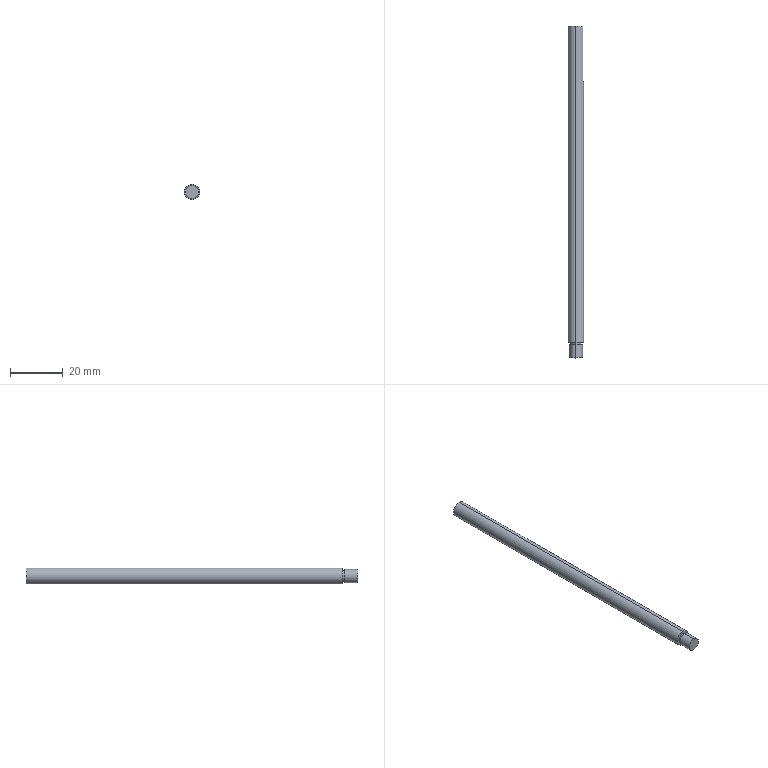Part | STEP file | 1 solid | 12 faces | box 6 x 126 x 6 mm | volume 3480 mm3 | cylinder 6 | plane 6 | commonest cylinder face diameters 4 x2 5 x2 6 x2
STEP:
#1=CARTESIAN_POINT('',(0.,0.,0.));
#2=DIRECTION('',(0.,0.,1.));
#3=DIRECTION('',(1.,0.,0.));
#4=AXIS2_PLACEMENT_3D('',#1,#2,#3);
#5=CARTESIAN_POINT('',(0.,-6.,-2.5));
#6=VERTEX_POINT('',#5);
#7=CARTESIAN_POINT('',(0.,-6.,2.5));
#8=VERTEX_POINT('',#7);
#9=CARTESIAN_POINT('',(0.,-6.,0.));
#10=DIRECTION('',(0.,-1.,0.));
#11=DIRECTION('',(0.,0.,-1.));
#12=AXIS2_PLACEMENT_3D('',#9,#10,#11);
#13=CIRCLE('',#12,2.5);
#14=CARTESIAN_POINT('',(0.,-6.,0.));
#15=DIRECTION('',(0.,1.,0.));
#16=DIRECTION('',(0.,0.,1.));
#17=AXIS2_PLACEMENT_3D('',#14,#15,#16);
#18=CYLINDRICAL_SURFACE('',#17,2.5);
#19=CARTESIAN_POINT('',(3.142,0.));
#20=DIRECTION('',(-1.,0.));
#21=VECTOR('',#20,1.);
#22=LINE('',#19,#21);
#23=(GEOMETRIC_REPRESENTATION_CONTEXT(2)PARAMETRIC_REPRESENTATION_CONTEXT()REPRESENTATION_CONTEXT('',''));
#24=DEFINITIONAL_REPRESENTATION('',(#22),#23);
#25=PCURVE('',#18,#24);
#26=CARTESIAN_POINT('',(0.,-6.,0.));
#27=DIRECTION('',(0.,-1.,0.));
#28=DIRECTION('',(0.,0.,-1.));
#29=AXIS2_PLACEMENT_3D('',#26,#27,#28);
#30=PLANE('',#29);
#31=CARTESIAN_POINT('',(0.,0.));
#32=DIRECTION('',(1.,0.));
#33=AXIS2_PLACEMENT_2D('',#31,#32);
#34=CIRCLE('',#33,2.5);
#35=(GEOMETRIC_REPRESENTATION_CONTEXT(2)PARAMETRIC_REPRESENTATION_CONTEXT()REPRESENTATION_CONTEXT('',''));
#36=DEFINITIONAL_REPRESENTATION('',(#34),#35);
#37=PCURVE('',#30,#36);
#38=SURFACE_CURVE('',#13,(#25,#37),.PCURVE_S1.);
#39=EDGE_CURVE('',#6,#8,#38,.T.);
#40=ORIENTED_EDGE('',*,*,#39,.F.);
#41=CARTESIAN_POINT('',(0.,-1.,-2.5));
#42=VERTEX_POINT('',#41);
#43=CARTESIAN_POINT('',(0.,-6.,-2.5));
#44=DIRECTION('',(0.,1.,0.));
#45=VECTOR('',#44,1.);
#46=LINE('',#43,#45);
#47=CARTESIAN_POINT('',(3.142,0.));
#48=DIRECTION('',(0.,1.));
#49=VECTOR('',#48,1.);
#50=LINE('',#47,#49);
#51=(GEOMETRIC_REPRESENTATION_CONTEXT(2)PARAMETRIC_REPRESENTATION_CONTEXT()REPRESENTATION_CONTEXT('',''));
#52=DEFINITIONAL_REPRESENTATION('',(#50),#51);
#53=PCURVE('',#18,#52);
#54=CARTESIAN_POINT('',(0.,-6.,0.));
#55=DIRECTION('',(0.,1.,0.));
#56=DIRECTION('',(0.,0.,1.));
#57=AXIS2_PLACEMENT_3D('',#54,#55,#56);
#58=CYLINDRICAL_SURFACE('',#57,2.5);
#59=CARTESIAN_POINT('',(3.142,0.));
#60=DIRECTION('',(0.,1.));
#61=VECTOR('',#60,1.);
#62=LINE('',#59,#61);
#63=(GEOMETRIC_REPRESENTATION_CONTEXT(2)PARAMETRIC_REPRESENTATION_CONTEXT()REPRESENTATION_CONTEXT('',''));
#64=DEFINITIONAL_REPRESENTATION('',(#62),#63);
#65=PCURVE('',#58,#64);
#66=SURFACE_CURVE('',#46,(#53,#65),.PCURVE_S1.);
#67=EDGE_CURVE('',#6,#42,#66,.T.);
#68=ORIENTED_EDGE('',*,*,#67,.T.);
#69=CARTESIAN_POINT('',(0.,-1.,2.5));
#70=VERTEX_POINT('',#69);
#71=CARTESIAN_POINT('',(0.,-1.,0.));
#72=DIRECTION('',(0.,-1.,0.));
#73=DIRECTION('',(0.,0.,-1.));
#74=AXIS2_PLACEMENT_3D('',#71,#72,#73);
#75=CIRCLE('',#74,2.5);
#76=CARTESIAN_POINT('',(3.142,5.));
#77=DIRECTION('',(-1.,0.));
#78=VECTOR('',#77,1.);
#79=LINE('',#76,#78);
#80=(GEOMETRIC_REPRESENTATION_CONTEXT(2)PARAMETRIC_REPRESENTATION_CONTEXT()REPRESENTATION_CONTEXT('',''));
#81=DEFINITIONAL_REPRESENTATION('',(#79),#80);
#82=PCURVE('',#18,#81);
#83=CARTESIAN_POINT('',(0.,-1.,0.));
#84=DIRECTION('',(0.,-1.,0.));
#85=DIRECTION('',(0.,0.,-1.));
#86=AXIS2_PLACEMENT_3D('',#83,#84,#85);
#87=PLANE('',#86);
#88=CARTESIAN_POINT('',(0.,0.));
#89=DIRECTION('',(1.,0.));
#90=AXIS2_PLACEMENT_2D('',#88,#89);
#91=CIRCLE('',#90,2.5);
#92=(GEOMETRIC_REPRESENTATION_CONTEXT(2)PARAMETRIC_REPRESENTATION_CONTEXT()REPRESENTATION_CONTEXT('',''));
#93=DEFINITIONAL_REPRESENTATION('',(#91),#92);
#94=PCURVE('',#87,#93);
#95=SURFACE_CURVE('',#75,(#82,#94),.PCURVE_S1.);
#96=EDGE_CURVE('',#42,#70,#95,.T.);
#97=ORIENTED_EDGE('',*,*,#96,.T.);
#98=CARTESIAN_POINT('',(0.,-6.,2.5));
#99=DIRECTION('',(0.,1.,0.));
#100=VECTOR('',#99,1.);
#101=LINE('',#98,#100);
#102=CARTESIAN_POINT('',(0.,0.));
#103=DIRECTION('',(0.,1.));
#104=VECTOR('',#103,1.);
#105=LINE('',#102,#104);
#106=(GEOMETRIC_REPRESENTATION_CONTEXT(2)PARAMETRIC_REPRESENTATION_CONTEXT()REPRESENTATION_CONTEXT('',''));
#107=DEFINITIONAL_REPRESENTATION('',(#105),#106);
#108=PCURVE('',#18,#107);
#109=CARTESIAN_POINT('',(6.283,0.));
#110=DIRECTION('',(0.,1.));
#111=VECTOR('',#110,1.);
#112=LINE('',#109,#111);
#113=(GEOMETRIC_REPRESENTATION_CONTEXT(2)PARAMETRIC_REPRESENTATION_CONTEXT()REPRESENTATION_CONTEXT('',''));
#114=DEFINITIONAL_REPRESENTATION('',(#112),#113);
#115=PCURVE('',#58,#114);
#116=SURFACE_CURVE('',#101,(#108,#115),.PCURVE_S1.);
#117=EDGE_CURVE('',#8,#70,#116,.T.);
#118=ORIENTED_EDGE('',*,*,#117,.F.);
#119=EDGE_LOOP('',(#40,#68,#97,#118));
#120=FACE_BOUND('',#119,.T.);
#121=ADVANCED_FACE('',(#120),#18,.T.);
#122=CARTESIAN_POINT('',(0.,-1.,-2.));
#123=VERTEX_POINT('',#122);
#124=CARTESIAN_POINT('',(0.,-1.,2.));
#125=VERTEX_POINT('',#124);
#126=CARTESIAN_POINT('',(0.,-1.,0.));
#127=DIRECTION('',(0.,-1.,0.));
#128=DIRECTION('',(0.,0.,-1.));
#129=AXIS2_PLACEMENT_3D('',#126,#127,#128);
#130=CIRCLE('',#129,2.);
#131=CARTESIAN_POINT('',(0.,-1.,0.));
#132=DIRECTION('',(0.,1.,0.));
#133=DIRECTION('',(0.,0.,1.));
#134=AXIS2_PLACEMENT_3D('',#131,#132,#133);
#135=CYLINDRICAL_SURFACE('',#134,2.);
#136=CARTESIAN_POINT('',(3.142,0.));
#137=DIRECTION('',(-1.,0.));
#138=VECTOR('',#137,1.);
#139=LINE('',#136,#138);
#140=(GEOMETRIC_REPRESENTATION_CONTEXT(2)PARAMETRIC_REPRESENTATION_CONTEXT()REPRESENTATION_CONTEXT('',''));
#141=DEFINITIONAL_REPRESENTATION('',(#139),#140);
#142=PCURVE('',#135,#141);
#143=CARTESIAN_POINT('',(0.,0.));
#144=DIRECTION('',(1.,0.));
#145=AXIS2_PLACEMENT_2D('',#143,#144);
#146=CIRCLE('',#145,2.);
#147=(GEOMETRIC_REPRESENTATION_CONTEXT(2)PARAMETRIC_REPRESENTATION_CONTEXT()REPRESENTATION_CONTEXT('',''));
#148=DEFINITIONAL_REPRESENTATION('',(#146),#147);
#149=PCURVE('',#87,#148);
#150=SURFACE_CURVE('',#130,(#142,#149),.PCURVE_S1.);
#151=EDGE_CURVE('',#123,#125,#150,.T.);
#152=ORIENTED_EDGE('',*,*,#151,.F.);
#153=CARTESIAN_POINT('',(0.,0.,-2.));
#154=VERTEX_POINT('',#153);
#155=CARTESIAN_POINT('',(0.,-1.,-2.));
#156=DIRECTION('',(0.,1.,0.));
#157=VECTOR('',#156,1.);
#158=LINE('',#155,#157);
#159=CARTESIAN_POINT('',(3.142,0.));
#160=DIRECTION('',(0.,1.));
#161=VECTOR('',#160,1.);
#162=LINE('',#159,#161);
#163=(GEOMETRIC_REPRESENTATION_CONTEXT(2)PARAMETRIC_REPRESENTATION_CONTEXT()REPRESENTATION_CONTEXT('',''));
#164=DEFINITIONAL_REPRESENTATION('',(#162),#163);
#165=PCURVE('',#135,#164);
#166=CARTESIAN_POINT('',(0.,-1.,0.));
#167=DIRECTION('',(0.,1.,0.));
#168=DIRECTION('',(0.,0.,1.));
#169=AXIS2_PLACEMENT_3D('',#166,#167,#168);
#170=CYLINDRICAL_SURFACE('',#169,2.);
#171=CARTESIAN_POINT('',(3.142,0.));
#172=DIRECTION('',(0.,1.));
#173=VECTOR('',#172,1.);
#174=LINE('',#171,#173);
#175=(GEOMETRIC_REPRESENTATION_CONTEXT(2)PARAMETRIC_REPRESENTATION_CONTEXT()REPRESENTATION_CONTEXT('',''));
#176=DEFINITIONAL_REPRESENTATION('',(#174),#175);
#177=PCURVE('',#170,#176);
#178=SURFACE_CURVE('',#158,(#165,#177),.PCURVE_S1.);
#179=EDGE_CURVE('',#123,#154,#178,.T.);
#180=ORIENTED_EDGE('',*,*,#179,.T.);
#181=CARTESIAN_POINT('',(0.,0.,2.));
#182=VERTEX_POINT('',#181);
#183=CARTESIAN_POINT('',(0.,0.,0.));
#184=DIRECTION('',(0.,-1.,0.));
#185=DIRECTION('',(0.,0.,-1.));
#186=AXIS2_PLACEMENT_3D('',#183,#184,#185);
#187=CIRCLE('',#186,2.);
#188=CARTESIAN_POINT('',(3.142,1.));
#189=DIRECTION('',(-1.,0.));
#190=VECTOR('',#189,1.);
#191=LINE('',#188,#190);
#192=(GEOMETRIC_REPRESENTATION_CONTEXT(2)PARAMETRIC_REPRESENTATION_CONTEXT()REPRESENTATION_CONTEXT('',''));
#193=DEFINITIONAL_REPRESENTATION('',(#191),#192);
#194=PCURVE('',#135,#193);
#195=CARTESIAN_POINT('',(0.,0.,0.));
#196=DIRECTION('',(0.,1.,0.));
#197=DIRECTION('',(0.,0.,1.));
#198=AXIS2_PLACEMENT_3D('',#195,#196,#197);
#199=PLANE('',#198);
#200=CARTESIAN_POINT('',(-2.,0.));
#201=CARTESIAN_POINT('',(-2.,3.464));
#202=CARTESIAN_POINT('',(1.,1.732));
#203=CARTESIAN_POINT('',(4.,0.));
#204=CARTESIAN_POINT('',(1.,-1.732));
#205=CARTESIAN_POINT('',(-2.,-3.464));
#206=CARTESIAN_POINT('',(-2.,0.));
#207=(BOUNDED_CURVE()B_SPLINE_CURVE(2,(#200,#201,#202,#203,#204,#205,#206),.UNSPECIFIED.,.T.,.F.)B_SPLINE_CURVE_WITH_KNOTS((1,2,2,2,2,1),(-2.094,0.,2.094,4.189,6.283,8.378),.UNSPECIFIED.)CURVE()GEOMETRIC_REPRESENTATION_ITEM()RATIONAL_B_SPLINE_CURVE((1.,0.5,1.,0.5,1.,0.5,1.))REPRESENTATION_ITEM(''));
#208=(GEOMETRIC_REPRESENTATION_CONTEXT(2)PARAMETRIC_REPRESENTATION_CONTEXT()REPRESENTATION_CONTEXT('',''));
#209=DEFINITIONAL_REPRESENTATION('',(#207),#208);
#210=PCURVE('',#199,#209);
#211=SURFACE_CURVE('',#187,(#194,#210),.PCURVE_S1.);
#212=EDGE_CURVE('',#154,#182,#211,.T.);
#213=ORIENTED_EDGE('',*,*,#212,.T.);
#214=CARTESIAN_POINT('',(0.,-1.,2.));
#215=DIRECTION('',(0.,1.,0.));
#216=VECTOR('',#215,1.);
#217=LINE('',#214,#216);
#218=CARTESIAN_POINT('',(0.,0.));
#219=DIRECTION('',(0.,1.));
#220=VECTOR('',#219,1.);
#221=LINE('',#218,#220);
#222=(GEOMETRIC_REPRESENTATION_CONTEXT(2)PARAMETRIC_REPRESENTATION_CONTEXT()REPRESENTATION_CONTEXT('',''));
#223=DEFINITIONAL_REPRESENTATION('',(#221),#222);
#224=PCURVE('',#135,#223);
#225=CARTESIAN_POINT('',(6.283,0.));
#226=DIRECTION('',(0.,1.));
#227=VECTOR('',#226,1.);
#228=LINE('',#225,#227);
#229=(GEOMETRIC_REPRESENTATION_CONTEXT(2)PARAMETRIC_REPRESENTATION_CONTEXT()REPRESENTATION_CONTEXT('',''));
#230=DEFINITIONAL_REPRESENTATION('',(#228),#229);
#231=PCURVE('',#170,#230);
#232=SURFACE_CURVE('',#217,(#224,#231),.PCURVE_S1.);
#233=EDGE_CURVE('',#125,#182,#232,.T.);
#234=ORIENTED_EDGE('',*,*,#233,.F.);
#235=EDGE_LOOP('',(#152,#180,#213,#234));
#236=FACE_BOUND('',#235,.T.);
#237=ADVANCED_FACE('',(#236),#135,.T.);
#238=CARTESIAN_POINT('',(0.,120.,3.));
#239=VERTEX_POINT('',#238);
#240=CARTESIAN_POINT('',(2.5,120.,1.658));
#241=VERTEX_POINT('',#240);
#242=CARTESIAN_POINT('',(0.,120.,0.));
#243=DIRECTION('',(0.,1.,0.));
#244=DIRECTION('',(0.,0.,1.));
#245=AXIS2_PLACEMENT_3D('',#242,#243,#244);
#246=CIRCLE('',#245,3.);
#247=CARTESIAN_POINT('',(0.,120.,0.));
#248=DIRECTION('',(0.,-1.,0.));
#249=DIRECTION('',(0.,0.,-1.));
#250=AXIS2_PLACEMENT_3D('',#247,#248,#249);
#251=CYLINDRICAL_SURFACE('',#250,3.);
#252=CARTESIAN_POINT('',(3.142,0.));
#253=DIRECTION('',(-1.,0.));
#254=VECTOR('',#253,1.);
#255=LINE('',#252,#254);
#256=(GEOMETRIC_REPRESENTATION_CONTEXT(2)PARAMETRIC_REPRESENTATION_CONTEXT()REPRESENTATION_CONTEXT('',''));
#257=DEFINITIONAL_REPRESENTATION('',(#255),#256);
#258=PCURVE('',#251,#257);
#259=CARTESIAN_POINT('',(0.,120.,0.));
#260=DIRECTION('',(0.,1.,0.));
#261=DIRECTION('',(0.,0.,1.));
#262=AXIS2_PLACEMENT_3D('',#259,#260,#261);
#263=PLANE('',#262);
#264=CARTESIAN_POINT('',(0.,0.));
#265=DIRECTION('',(1.,0.));
#266=AXIS2_PLACEMENT_2D('',#264,#265);
#267=CIRCLE('',#266,3.);
#268=(GEOMETRIC_REPRESENTATION_CONTEXT(2)PARAMETRIC_REPRESENTATION_CONTEXT()REPRESENTATION_CONTEXT('',''));
#269=DEFINITIONAL_REPRESENTATION('',(#267),#268);
#270=PCURVE('',#263,#269);
#271=SURFACE_CURVE('',#246,(#258,#270),.PCURVE_S1.);
#272=EDGE_CURVE('',#239,#241,#271,.T.);
#273=ORIENTED_EDGE('',*,*,#272,.F.);
#274=CARTESIAN_POINT('',(0.,0.,3.));
#275=VERTEX_POINT('',#274);
#276=CARTESIAN_POINT('',(0.,120.,3.));
#277=DIRECTION('',(0.,-1.,0.));
#278=VECTOR('',#277,1.);
#279=LINE('',#276,#278);
#280=CARTESIAN_POINT('',(3.142,0.));
#281=DIRECTION('',(0.,1.));
#282=VECTOR('',#281,1.);
#283=LINE('',#280,#282);
#284=(GEOMETRIC_REPRESENTATION_CONTEXT(2)PARAMETRIC_REPRESENTATION_CONTEXT()REPRESENTATION_CONTEXT('',''));
#285=DEFINITIONAL_REPRESENTATION('',(#283),#284);
#286=PCURVE('',#251,#285);
#287=CARTESIAN_POINT('',(0.,120.,0.));
#288=DIRECTION('',(0.,-1.,0.));
#289=DIRECTION('',(0.,0.,-1.));
#290=AXIS2_PLACEMENT_3D('',#287,#288,#289);
#291=CYLINDRICAL_SURFACE('',#290,3.);
#292=CARTESIAN_POINT('',(3.142,0.));
#293=DIRECTION('',(0.,1.));
#294=VECTOR('',#293,1.);
#295=LINE('',#292,#294);
#296=(GEOMETRIC_REPRESENTATION_CONTEXT(2)PARAMETRIC_REPRESENTATION_CONTEXT()REPRESENTATION_CONTEXT('',''));
#297=DEFINITIONAL_REPRESENTATION('',(#295),#296);
#298=PCURVE('',#291,#297);
#299=SURFACE_CURVE('',#279,(#286,#298),.PCURVE_S1.);
#300=EDGE_CURVE('',#239,#275,#299,.T.);
#301=ORIENTED_EDGE('',*,*,#300,.T.);
#302=CARTESIAN_POINT('',(0.,0.,-3.));
#303=VERTEX_POINT('',#302);
#304=CARTESIAN_POINT('',(0.,0.,0.));
#305=DIRECTION('',(0.,1.,0.));
#306=DIRECTION('',(0.,0.,1.));
#307=AXIS2_PLACEMENT_3D('',#304,#305,#306);
#308=CIRCLE('',#307,3.);
#309=CARTESIAN_POINT('',(3.142,120.));
#310=DIRECTION('',(-1.,0.));
#311=VECTOR('',#310,1.);
#312=LINE('',#309,#311);
#313=(GEOMETRIC_REPRESENTATION_CONTEXT(2)PARAMETRIC_REPRESENTATION_CONTEXT()REPRESENTATION_CONTEXT('',''));
#314=DEFINITIONAL_REPRESENTATION('',(#312),#313);
#315=PCURVE('',#251,#314);
#316=CARTESIAN_POINT('',(0.,0.));
#317=DIRECTION('',(1.,0.));
#318=AXIS2_PLACEMENT_2D('',#316,#317);
#319=CIRCLE('',#318,3.);
#320=(GEOMETRIC_REPRESENTATION_CONTEXT(2)PARAMETRIC_REPRESENTATION_CONTEXT()REPRESENTATION_CONTEXT('',''));
#321=DEFINITIONAL_REPRESENTATION('',(#319),#320);
#322=PCURVE('',#199,#321);
#323=SURFACE_CURVE('',#308,(#315,#322),.PCURVE_S1.);
#324=EDGE_CURVE('',#275,#303,#323,.T.);
#325=ORIENTED_EDGE('',*,*,#324,.T.);
#326=CARTESIAN_POINT('',(0.,120.,-3.));
#327=VERTEX_POINT('',#326);
#328=CARTESIAN_POINT('',(0.,120.,-3.));
#329=DIRECTION('',(0.,-1.,0.));
#330=VECTOR('',#329,1.);
#331=LINE('',#328,#330);
#332=CARTESIAN_POINT('',(0.,0.));
#333=DIRECTION('',(0.,1.));
#334=VECTOR('',#333,1.);
#335=LINE('',#332,#334);
#336=(GEOMETRIC_REPRESENTATION_CONTEXT(2)PARAMETRIC_REPRESENTATION_CONTEXT()REPRESENTATION_CONTEXT('',''));
#337=DEFINITIONAL_REPRESENTATION('',(#335),#336);
#338=PCURVE('',#251,#337);
#339=CARTESIAN_POINT('',(6.283,0.));
#340=DIRECTION('',(0.,1.));
#341=VECTOR('',#340,1.);
#342=LINE('',#339,#341);
#343=(GEOMETRIC_REPRESENTATION_CONTEXT(2)PARAMETRIC_REPRESENTATION_CONTEXT()REPRESENTATION_CONTEXT('',''));
#344=DEFINITIONAL_REPRESENTATION('',(#342),#343);
#345=PCURVE('',#291,#344);
#346=SURFACE_CURVE('',#331,(#338,#345),.PCURVE_S1.);
#347=EDGE_CURVE('',#327,#303,#346,.T.);
#348=ORIENTED_EDGE('',*,*,#347,.F.);
#349=CARTESIAN_POINT('',(2.5,120.,-1.658));
#350=VERTEX_POINT('',#349);
#351=CARTESIAN_POINT('',(0.,120.,0.));
#352=DIRECTION('',(0.,1.,0.));
#353=DIRECTION('',(0.,0.,1.));
#354=AXIS2_PLACEMENT_3D('',#351,#352,#353);
#355=CIRCLE('',#354,3.);
#356=CARTESIAN_POINT('',(3.142,0.));
#357=DIRECTION('',(-1.,0.));
#358=VECTOR('',#357,1.);
#359=LINE('',#356,#358);
#360=(GEOMETRIC_REPRESENTATION_CONTEXT(2)PARAMETRIC_REPRESENTATION_CONTEXT()REPRESENTATION_CONTEXT('',''));
#361=DEFINITIONAL_REPRESENTATION('',(#359),#360);
#362=PCURVE('',#251,#361);
#363=CARTESIAN_POINT('',(0.,0.));
#364=DIRECTION('',(1.,0.));
#365=AXIS2_PLACEMENT_2D('',#363,#364);
#366=CIRCLE('',#365,3.);
#367=(GEOMETRIC_REPRESENTATION_CONTEXT(2)PARAMETRIC_REPRESENTATION_CONTEXT()REPRESENTATION_CONTEXT('',''));
#368=DEFINITIONAL_REPRESENTATION('',(#366),#367);
#369=PCURVE('',#263,#368);
#370=SURFACE_CURVE('',#355,(#362,#369),.PCURVE_S1.);
#371=EDGE_CURVE('',#350,#327,#370,.T.);
#372=ORIENTED_EDGE('',*,*,#371,.F.);
#373=CARTESIAN_POINT('',(2.5,99.,-1.658));
#374=VERTEX_POINT('',#373);
#375=CARTESIAN_POINT('',(2.5,120.,-1.658));
#376=DIRECTION('',(0.,-1.,0.));
#377=VECTOR('',#376,1.);
#378=LINE('',#375,#377);
#379=CARTESIAN_POINT('',(0.9851,0.));
#380=DIRECTION('',(0.,1.));
#381=VECTOR('',#380,1.);
#382=LINE('',#379,#381);
#383=(GEOMETRIC_REPRESENTATION_CONTEXT(2)PARAMETRIC_REPRESENTATION_CONTEXT()REPRESENTATION_CONTEXT('',''));
#384=DEFINITIONAL_REPRESENTATION('',(#382),#383);
#385=PCURVE('',#251,#384);
#386=CARTESIAN_POINT('',(2.5,120.,-3.));
#387=DIRECTION('',(-1.,0.,0.));
#388=DIRECTION('',(0.,-1.,0.));
#389=AXIS2_PLACEMENT_3D('',#386,#387,#388);
#390=PLANE('',#389);
#391=CARTESIAN_POINT('',(0.,1.342));
#392=DIRECTION('',(1.,0.));
#393=VECTOR('',#392,1.);
#394=LINE('',#391,#393);
#395=(GEOMETRIC_REPRESENTATION_CONTEXT(2)PARAMETRIC_REPRESENTATION_CONTEXT()REPRESENTATION_CONTEXT('',''));
#396=DEFINITIONAL_REPRESENTATION('',(#394),#395);
#397=PCURVE('',#390,#396);
#398=SURFACE_CURVE('',#378,(#385,#397),.PCURVE_S1.);
#399=EDGE_CURVE('',#350,#374,#398,.T.);
#400=ORIENTED_EDGE('',*,*,#399,.T.);
#401=CARTESIAN_POINT('',(2.5,99.,1.658));
#402=VERTEX_POINT('',#401);
#403=CARTESIAN_POINT('',(0.,99.,0.));
#404=DIRECTION('',(0.,-1.,0.));
#405=DIRECTION('',(0.,0.,-1.));
#406=AXIS2_PLACEMENT_3D('',#403,#404,#405);
#407=CIRCLE('',#406,3.);
#408=CARTESIAN_POINT('',(0.,21.));
#409=DIRECTION('',(1.,0.));
#410=VECTOR('',#409,1.);
#411=LINE('',#408,#410);
#412=(GEOMETRIC_REPRESENTATION_CONTEXT(2)PARAMETRIC_REPRESENTATION_CONTEXT()REPRESENTATION_CONTEXT('',''));
#413=DEFINITIONAL_REPRESENTATION('',(#411),#412);
#414=PCURVE('',#251,#413);
#415=CARTESIAN_POINT('',(3.,99.,-3.));
#416=DIRECTION('',(0.,-1.,0.));
#417=DIRECTION('',(0.,0.,-1.));
#418=AXIS2_PLACEMENT_3D('',#415,#416,#417);
#419=PLANE('',#418);
#420=CARTESIAN_POINT('',(-3.,-3.));
#421=DIRECTION('',(1.,0.));
#422=AXIS2_PLACEMENT_2D('',#420,#421);
#423=CIRCLE('',#422,3.);
#424=(GEOMETRIC_REPRESENTATION_CONTEXT(2)PARAMETRIC_REPRESENTATION_CONTEXT()REPRESENTATION_CONTEXT('',''));
#425=DEFINITIONAL_REPRESENTATION('',(#423),#424);
#426=PCURVE('',#419,#425);
#427=SURFACE_CURVE('',#407,(#414,#426),.PCURVE_S1.);
#428=EDGE_CURVE('',#374,#402,#427,.T.);
#429=ORIENTED_EDGE('',*,*,#428,.T.);
#430=CARTESIAN_POINT('',(2.5,120.,1.658));
#431=DIRECTION('',(0.,1.,0.));
#432=VECTOR('',#431,1.);
#433=LINE('',#430,#432);
#434=CARTESIAN_POINT('',(2.156,0.));
#435=DIRECTION('',(0.,-1.));
#436=VECTOR('',#435,1.);
#437=LINE('',#434,#436);
#438=(GEOMETRIC_REPRESENTATION_CONTEXT(2)PARAMETRIC_REPRESENTATION_CONTEXT()REPRESENTATION_CONTEXT('',''));
#439=DEFINITIONAL_REPRESENTATION('',(#437),#438);
#440=PCURVE('',#251,#439);
#441=CARTESIAN_POINT('',(0.,4.658));
#442=DIRECTION('',(-1.,0.));
#443=VECTOR('',#442,1.);
#444=LINE('',#441,#443);
#445=(GEOMETRIC_REPRESENTATION_CONTEXT(2)PARAMETRIC_REPRESENTATION_CONTEXT()REPRESENTATION_CONTEXT('',''));
#446=DEFINITIONAL_REPRESENTATION('',(#444),#445);
#447=PCURVE('',#390,#446);
#448=SURFACE_CURVE('',#433,(#440,#447),.PCURVE_S1.);
#449=EDGE_CURVE('',#402,#241,#448,.T.);
#450=ORIENTED_EDGE('',*,*,#449,.T.);
#451=EDGE_LOOP('',(#273,#301,#325,#348,#372,#400,#429,#450));
#452=FACE_BOUND('',#451,.T.);
#453=ADVANCED_FACE('',(#452),#251,.T.);
#454=ORIENTED_EDGE('',*,*,#300,.F.);
#455=CARTESIAN_POINT('',(0.,120.,0.));
#456=DIRECTION('',(0.,1.,0.));
#457=DIRECTION('',(0.,0.,1.));
#458=AXIS2_PLACEMENT_3D('',#455,#456,#457);
#459=CIRCLE('',#458,3.);
#460=CARTESIAN_POINT('',(9.425,0.));
#461=DIRECTION('',(-1.,0.));
#462=VECTOR('',#461,1.);
#463=LINE('',#460,#462);
#464=(GEOMETRIC_REPRESENTATION_CONTEXT(2)PARAMETRIC_REPRESENTATION_CONTEXT()REPRESENTATION_CONTEXT('',''));
#465=DEFINITIONAL_REPRESENTATION('',(#463),#464);
#466=PCURVE('',#291,#465);
#467=CARTESIAN_POINT('',(0.,0.));
#468=DIRECTION('',(1.,0.));
#469=AXIS2_PLACEMENT_2D('',#467,#468);
#470=CIRCLE('',#469,3.);
#471=(GEOMETRIC_REPRESENTATION_CONTEXT(2)PARAMETRIC_REPRESENTATION_CONTEXT()REPRESENTATION_CONTEXT('',''));
#472=DEFINITIONAL_REPRESENTATION('',(#470),#471);
#473=PCURVE('',#263,#472);
#474=SURFACE_CURVE('',#459,(#466,#473),.PCURVE_S1.);
#475=EDGE_CURVE('',#327,#239,#474,.T.);
#476=ORIENTED_EDGE('',*,*,#475,.F.);
#477=ORIENTED_EDGE('',*,*,#347,.T.);
#478=CARTESIAN_POINT('',(0.,0.,0.));
#479=DIRECTION('',(0.,1.,0.));
#480=DIRECTION('',(0.,0.,1.));
#481=AXIS2_PLACEMENT_3D('',#478,#479,#480);
#482=CIRCLE('',#481,3.);
#483=CARTESIAN_POINT('',(9.425,120.));
#484=DIRECTION('',(-1.,0.));
#485=VECTOR('',#484,1.);
#486=LINE('',#483,#485);
#487=(GEOMETRIC_REPRESENTATION_CONTEXT(2)PARAMETRIC_REPRESENTATION_CONTEXT()REPRESENTATION_CONTEXT('',''));
#488=DEFINITIONAL_REPRESENTATION('',(#486),#487);
#489=PCURVE('',#291,#488);
#490=CARTESIAN_POINT('',(0.,0.));
#491=DIRECTION('',(1.,0.));
#492=AXIS2_PLACEMENT_2D('',#490,#491);
#493=CIRCLE('',#492,3.);
#494=(GEOMETRIC_REPRESENTATION_CONTEXT(2)PARAMETRIC_REPRESENTATION_CONTEXT()REPRESENTATION_CONTEXT('',''));
#495=DEFINITIONAL_REPRESENTATION('',(#493),#494);
#496=PCURVE('',#199,#495);
#497=SURFACE_CURVE('',#482,(#489,#496),.PCURVE_S1.);
#498=EDGE_CURVE('',#303,#275,#497,.T.);
#499=ORIENTED_EDGE('',*,*,#498,.T.);
#500=EDGE_LOOP('',(#454,#476,#477,#499));
#501=FACE_BOUND('',#500,.T.);
#502=ADVANCED_FACE('',(#501),#291,.T.);
#503=CARTESIAN_POINT('',(2.5,120.,0.));
#504=DIRECTION('',(0.,0.,1.));
#505=VECTOR('',#504,1.);
#506=LINE('',#503,#505);
#507=CARTESIAN_POINT('',(0.,2.5));
#508=DIRECTION('',(1.,0.));
#509=VECTOR('',#508,1.);
#510=LINE('',#507,#509);
#511=(GEOMETRIC_REPRESENTATION_CONTEXT(2)PARAMETRIC_REPRESENTATION_CONTEXT()REPRESENTATION_CONTEXT('',''));
#512=DEFINITIONAL_REPRESENTATION('',(#510),#511);
#513=PCURVE('',#263,#512);
#514=CARTESIAN_POINT('',(0.,3.));
#515=DIRECTION('',(0.,1.));
#516=VECTOR('',#515,1.);
#517=LINE('',#514,#516);
#518=(GEOMETRIC_REPRESENTATION_CONTEXT(2)PARAMETRIC_REPRESENTATION_CONTEXT()REPRESENTATION_CONTEXT('',''));
#519=DEFINITIONAL_REPRESENTATION('',(#517),#518);
#520=PCURVE('',#390,#519);
#521=SURFACE_CURVE('',#506,(#513,#520),.PCURVE_S1.);
#522=EDGE_CURVE('',#350,#241,#521,.T.);
#523=ORIENTED_EDGE('',*,*,#522,.F.);
#524=ORIENTED_EDGE('',*,*,#371,.T.);
#525=ORIENTED_EDGE('',*,*,#475,.T.);
#526=ORIENTED_EDGE('',*,*,#272,.T.);
#527=EDGE_LOOP('',(#523,#524,#525,#526));
#528=FACE_BOUND('',#527,.T.);
#529=ADVANCED_FACE('',(#528),#263,.T.);
#530=ORIENTED_EDGE('',*,*,#498,.F.);
#531=ORIENTED_EDGE('',*,*,#324,.F.);
#532=EDGE_LOOP('',(#530,#531));
#533=FACE_BOUND('',#532,.T.);
#534=CARTESIAN_POINT('',(0.,0.,0.));
#535=DIRECTION('',(0.,-1.,0.));
#536=DIRECTION('',(0.,0.,-1.));
#537=AXIS2_PLACEMENT_3D('',#534,#535,#536);
#538=CIRCLE('',#537,2.);
#539=CARTESIAN_POINT('',(-2.,0.));
#540=CARTESIAN_POINT('',(-2.,3.464));
#541=CARTESIAN_POINT('',(1.,1.732));
#542=CARTESIAN_POINT('',(4.,0.));
#543=CARTESIAN_POINT('',(1.,-1.732));
#544=CARTESIAN_POINT('',(-2.,-3.464));
#545=CARTESIAN_POINT('',(-2.,0.));
#546=(BOUNDED_CURVE()B_SPLINE_CURVE(2,(#539,#540,#541,#542,#543,#544,#545),.UNSPECIFIED.,.T.,.F.)B_SPLINE_CURVE_WITH_KNOTS((1,2,2,2,2,1),(-2.094,0.,2.094,4.189,6.283,8.378),.UNSPECIFIED.)CURVE()GEOMETRIC_REPRESENTATION_ITEM()RATIONAL_B_SPLINE_CURVE((1.,0.5,1.,0.5,1.,0.5,1.))REPRESENTATION_ITEM(''));
#547=(GEOMETRIC_REPRESENTATION_CONTEXT(2)PARAMETRIC_REPRESENTATION_CONTEXT()REPRESENTATION_CONTEXT('',''));
#548=DEFINITIONAL_REPRESENTATION('',(#546),#547);
#549=PCURVE('',#199,#548);
#550=CARTESIAN_POINT('',(9.425,1.));
#551=DIRECTION('',(-1.,0.));
#552=VECTOR('',#551,1.);
#553=LINE('',#550,#552);
#554=(GEOMETRIC_REPRESENTATION_CONTEXT(2)PARAMETRIC_REPRESENTATION_CONTEXT()REPRESENTATION_CONTEXT('',''));
#555=DEFINITIONAL_REPRESENTATION('',(#553),#554);
#556=PCURVE('',#170,#555);
#557=SURFACE_CURVE('',#538,(#549,#556),.PCURVE_S1.);
#558=EDGE_CURVE('',#182,#154,#557,.T.);
#559=ORIENTED_EDGE('',*,*,#558,.F.);
#560=ORIENTED_EDGE('',*,*,#212,.F.);
#561=EDGE_LOOP('',(#559,#560));
#562=FACE_BOUND('',#561,.T.);
#563=ADVANCED_FACE('',(#533,#562),#199,.F.);
#564=CARTESIAN_POINT('',(2.5,99.,-3.));
#565=DIRECTION('',(0.,0.,1.));
#566=VECTOR('',#565,1.);
#567=LINE('',#564,#566);
#568=CARTESIAN_POINT('',(0.,-0.5));
#569=DIRECTION('',(-1.,0.));
#570=VECTOR('',#569,1.);
#571=LINE('',#568,#570);
#572=(GEOMETRIC_REPRESENTATION_CONTEXT(2)PARAMETRIC_REPRESENTATION_CONTEXT()REPRESENTATION_CONTEXT('',''));
#573=DEFINITIONAL_REPRESENTATION('',(#571),#572);
#574=PCURVE('',#419,#573);
#575=CARTESIAN_POINT('',(21.,0.));
#576=DIRECTION('',(0.,1.));
#577=VECTOR('',#576,1.);
#578=LINE('',#575,#577);
#579=(GEOMETRIC_REPRESENTATION_CONTEXT(2)PARAMETRIC_REPRESENTATION_CONTEXT()REPRESENTATION_CONTEXT('',''));
#580=DEFINITIONAL_REPRESENTATION('',(#578),#579);
#581=PCURVE('',#390,#580);
#582=SURFACE_CURVE('',#567,(#574,#581),.PCURVE_S1.);
#583=EDGE_CURVE('',#374,#402,#582,.T.);
#584=ORIENTED_EDGE('',*,*,#583,.T.);
#585=ORIENTED_EDGE('',*,*,#428,.F.);
#586=EDGE_LOOP('',(#584,#585));
#587=FACE_BOUND('',#586,.T.);
#588=ADVANCED_FACE('',(#587),#419,.F.);
#589=ORIENTED_EDGE('',*,*,#522,.T.);
#590=ORIENTED_EDGE('',*,*,#449,.F.);
#591=ORIENTED_EDGE('',*,*,#583,.F.);
#592=ORIENTED_EDGE('',*,*,#399,.F.);
#593=EDGE_LOOP('',(#589,#590,#591,#592));
#594=FACE_BOUND('',#593,.T.);
#595=ADVANCED_FACE('',(#594),#390,.F.);
#596=CARTESIAN_POINT('',(0.,-1.,0.));
#597=DIRECTION('',(0.,-1.,0.));
#598=DIRECTION('',(0.,0.,-1.));
#599=AXIS2_PLACEMENT_3D('',#596,#597,#598);
#600=CIRCLE('',#599,2.5);
#601=CARTESIAN_POINT('',(0.,0.));
#602=DIRECTION('',(1.,0.));
#603=AXIS2_PLACEMENT_2D('',#601,#602);
#604=CIRCLE('',#603,2.5);
#605=(GEOMETRIC_REPRESENTATION_CONTEXT(2)PARAMETRIC_REPRESENTATION_CONTEXT()REPRESENTATION_CONTEXT('',''));
#606=DEFINITIONAL_REPRESENTATION('',(#604),#605);
#607=PCURVE('',#87,#606);
#608=CARTESIAN_POINT('',(9.425,5.));
#609=DIRECTION('',(-1.,0.));
#610=VECTOR('',#609,1.);
#611=LINE('',#608,#610);
#612=(GEOMETRIC_REPRESENTATION_CONTEXT(2)PARAMETRIC_REPRESENTATION_CONTEXT()REPRESENTATION_CONTEXT('',''));
#613=DEFINITIONAL_REPRESENTATION('',(#611),#612);
#614=PCURVE('',#58,#613);
#615=SURFACE_CURVE('',#600,(#607,#614),.PCURVE_S1.);
#616=EDGE_CURVE('',#70,#42,#615,.T.);
#617=ORIENTED_EDGE('',*,*,#616,.F.);
#618=ORIENTED_EDGE('',*,*,#96,.F.);
#619=EDGE_LOOP('',(#617,#618));
#620=FACE_BOUND('',#619,.T.);
#621=CARTESIAN_POINT('',(0.,-1.,0.));
#622=DIRECTION('',(0.,-1.,0.));
#623=DIRECTION('',(0.,0.,-1.));
#624=AXIS2_PLACEMENT_3D('',#621,#622,#623);
#625=CIRCLE('',#624,2.);
#626=CARTESIAN_POINT('',(0.,0.));
#627=DIRECTION('',(1.,0.));
#628=AXIS2_PLACEMENT_2D('',#626,#627);
#629=CIRCLE('',#628,2.);
#630=(GEOMETRIC_REPRESENTATION_CONTEXT(2)PARAMETRIC_REPRESENTATION_CONTEXT()REPRESENTATION_CONTEXT('',''));
#631=DEFINITIONAL_REPRESENTATION('',(#629),#630);
#632=PCURVE('',#87,#631);
#633=CARTESIAN_POINT('',(9.425,0.));
#634=DIRECTION('',(-1.,0.));
#635=VECTOR('',#634,1.);
#636=LINE('',#633,#635);
#637=(GEOMETRIC_REPRESENTATION_CONTEXT(2)PARAMETRIC_REPRESENTATION_CONTEXT()REPRESENTATION_CONTEXT('',''));
#638=DEFINITIONAL_REPRESENTATION('',(#636),#637);
#639=PCURVE('',#170,#638);
#640=SURFACE_CURVE('',#625,(#632,#639),.PCURVE_S1.);
#641=EDGE_CURVE('',#125,#123,#640,.T.);
#642=ORIENTED_EDGE('',*,*,#641,.T.);
#643=ORIENTED_EDGE('',*,*,#151,.T.);
#644=EDGE_LOOP('',(#642,#643));
#645=FACE_BOUND('',#644,.T.);
#646=ADVANCED_FACE('',(#620,#645),#87,.F.);
#647=ORIENTED_EDGE('',*,*,#179,.F.);
#648=ORIENTED_EDGE('',*,*,#641,.F.);
#649=ORIENTED_EDGE('',*,*,#233,.T.);
#650=ORIENTED_EDGE('',*,*,#558,.T.);
#651=EDGE_LOOP('',(#647,#648,#649,#650));
#652=FACE_BOUND('',#651,.T.);
#653=ADVANCED_FACE('',(#652),#170,.T.);
#654=CARTESIAN_POINT('',(0.,-6.,0.));
#655=DIRECTION('',(0.,-1.,0.));
#656=DIRECTION('',(0.,0.,-1.));
#657=AXIS2_PLACEMENT_3D('',#654,#655,#656);
#658=CIRCLE('',#657,2.5);
#659=CARTESIAN_POINT('',(0.,0.));
#660=DIRECTION('',(1.,0.));
#661=AXIS2_PLACEMENT_2D('',#659,#660);
#662=CIRCLE('',#661,2.5);
#663=(GEOMETRIC_REPRESENTATION_CONTEXT(2)PARAMETRIC_REPRESENTATION_CONTEXT()REPRESENTATION_CONTEXT('',''));
#664=DEFINITIONAL_REPRESENTATION('',(#662),#663);
#665=PCURVE('',#30,#664);
#666=CARTESIAN_POINT('',(9.425,0.));
#667=DIRECTION('',(-1.,0.));
#668=VECTOR('',#667,1.);
#669=LINE('',#666,#668);
#670=(GEOMETRIC_REPRESENTATION_CONTEXT(2)PARAMETRIC_REPRESENTATION_CONTEXT()REPRESENTATION_CONTEXT('',''));
#671=DEFINITIONAL_REPRESENTATION('',(#669),#670);
#672=PCURVE('',#58,#671);
#673=SURFACE_CURVE('',#658,(#665,#672),.PCURVE_S1.);
#674=EDGE_CURVE('',#8,#6,#673,.T.);
#675=ORIENTED_EDGE('',*,*,#674,.T.);
#676=ORIENTED_EDGE('',*,*,#39,.T.);
#677=EDGE_LOOP('',(#675,#676));
#678=FACE_BOUND('',#677,.T.);
#679=ADVANCED_FACE('',(#678),#30,.T.);
#680=ORIENTED_EDGE('',*,*,#67,.F.);
#681=ORIENTED_EDGE('',*,*,#674,.F.);
#682=ORIENTED_EDGE('',*,*,#117,.T.);
#683=ORIENTED_EDGE('',*,*,#616,.T.);
#684=EDGE_LOOP('',(#680,#681,#682,#683));
#685=FACE_BOUND('',#684,.T.);
#686=ADVANCED_FACE('',(#685),#58,.T.);
#687=CLOSED_SHELL('',(#121,#237,#453,#502,#529,#563,#588,#595,#646,#653,#679,#686));
#688=MANIFOLD_SOLID_BREP('',#687);
#689=(LENGTH_UNIT()NAMED_UNIT(*)SI_UNIT(.MILLI.,.METRE.));
#690=UNCERTAINTY_MEASURE_WITH_UNIT(LENGTH_MEASURE(0.0000001),#689,'','');
#691=(NAMED_UNIT(*)PLANE_ANGLE_UNIT()SI_UNIT($,.RADIAN.));
#692=(NAMED_UNIT(*)SI_UNIT($,.STERADIAN.)SOLID_ANGLE_UNIT());
#693=(GEOMETRIC_REPRESENTATION_CONTEXT(3)GLOBAL_UNCERTAINTY_ASSIGNED_CONTEXT((#690))GLOBAL_UNIT_ASSIGNED_CONTEXT((#689,#691,#692))REPRESENTATION_CONTEXT('',''));
#694=ADVANCED_BREP_SHAPE_REPRESENTATION('',(#4,#688),#693);